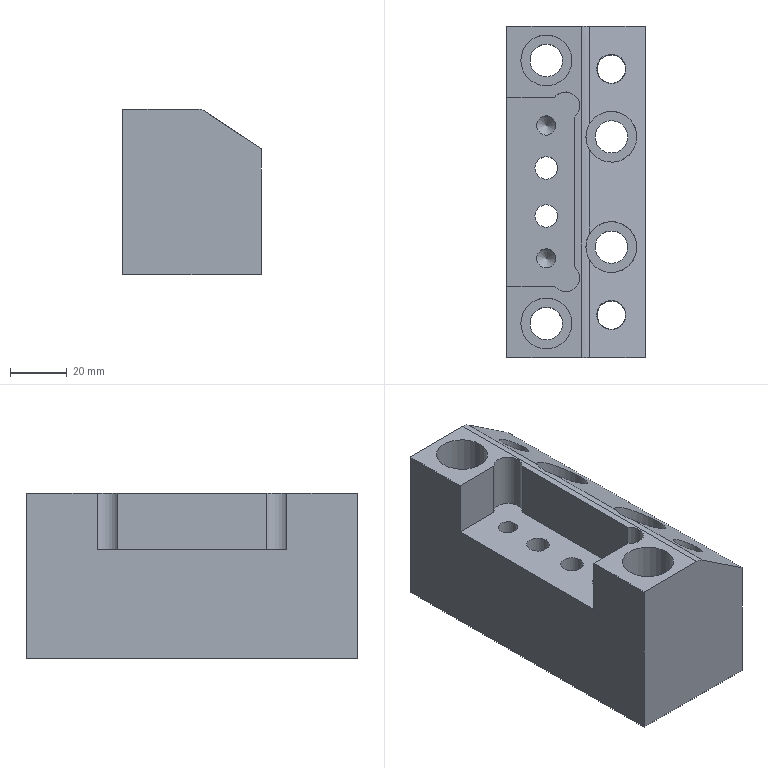Part | NX | features solid 2 | 1 solid | 42 faces | box 49 x 117 x 58.5 mm | volume 232068 mm3 | cylinder 21 | plane 19 | cone 2 | commonest cylinder face diameters 10 x5 11.5 x4 18 x4 6.8 x2 8.001 x2 10.001 x2
STEP:
#1=CARTESIAN_POINT('',(808.728,40.375,-5.567));
#2=VERTEX_POINT('',#1);
#3=CARTESIAN_POINT('',(813.878,40.375,-9.));
#4=DIRECTION('',(-0.5547,0.,-0.8321));
#5=DIRECTION('',(-0.8321,0.,0.5547));
#6=AXIS2_PLACEMENT_3D('',#3,#4,#5);
#7=ELLIPSE('',#6,6.19,5.15);
#8=EDGE_CURVE('',#2,#2,#7,.F.);
#9=ORIENTED_EDGE('',*,*,#8,.T.);
#10=EDGE_LOOP('',(#9));
#11=FACE_BOUND('',#10,.T.);
#12=CARTESIAN_POINT('',(808.728,40.375,-31.5));
#13=VERTEX_POINT('',#12);
#14=CARTESIAN_POINT('',(813.878,40.375,-31.5));
#15=DIRECTION('',(0.,0.,-1.));
#16=DIRECTION('',(-1.,0.,0.));
#17=AXIS2_PLACEMENT_3D('',#14,#15,#16);
#18=CIRCLE('',#17,5.15);
#19=EDGE_CURVE('',#13,#13,#18,.T.);
#20=ORIENTED_EDGE('',*,*,#19,.T.);
#21=EDGE_LOOP('',(#20));
#22=FACE_BOUND('',#21,.T.);
#23=CARTESIAN_POINT('',(813.878,40.375,-31.5));
#24=DIRECTION('',(0.,0.,1.));
#25=DIRECTION('',(1.,0.,0.));
#26=AXIS2_PLACEMENT_3D('',#23,#24,#25);
#27=CYLINDRICAL_SURFACE('',#26,5.15);
#28=ADVANCED_FACE('',(#11,#22),#27,.F.);
#29=ORIENTED_EDGE('',*,*,#19,.F.);
#30=EDGE_LOOP('',(#29));
#31=FACE_BOUND('',#30,.T.);
#32=CARTESIAN_POINT('',(808.877,40.375,-31.5));
#33=VERTEX_POINT('',#32);
#34=CARTESIAN_POINT('',(813.878,40.375,-31.5));
#35=DIRECTION('',(0.,0.,-1.));
#36=DIRECTION('',(-1.,0.,0.));
#37=AXIS2_PLACEMENT_3D('',#34,#35,#36);
#38=CIRCLE('',#37,5.);
#39=EDGE_CURVE('',#33,#33,#38,.F.);
#40=ORIENTED_EDGE('',*,*,#39,.F.);
#41=EDGE_LOOP('',(#40));
#42=FACE_BOUND('',#41,.T.);
#43=CARTESIAN_POINT('',(813.878,40.375,-31.5));
#44=DIRECTION('',(0.,0.,-1.));
#45=DIRECTION('',(-1.,0.,0.));
#46=AXIS2_PLACEMENT_3D('',#43,#44,#45);
#47=PLANE('',#46);
#48=ADVANCED_FACE('',(#31,#42),#47,.F.);
#49=CARTESIAN_POINT('',(795.878,5.375,-61.5));
#50=VERTEX_POINT('',#49);
#51=CARTESIAN_POINT('',(790.878,5.375,-61.5));
#52=DIRECTION('',(0.,0.,1.));
#53=DIRECTION('',(1.,0.,0.));
#54=AXIS2_PLACEMENT_3D('',#51,#52,#53);
#55=CIRCLE('',#54,5.);
#56=EDGE_CURVE('',#50,#50,#55,.F.);
#57=ORIENTED_EDGE('',*,*,#56,.F.);
#58=EDGE_LOOP('',(#57));
#59=FACE_BOUND('',#58,.T.);
#60=CARTESIAN_POINT('',(795.878,-11.625,-61.5));
#61=VERTEX_POINT('',#60);
#62=CARTESIAN_POINT('',(790.878,-11.625,-61.5));
#63=DIRECTION('',(0.,0.,1.));
#64=DIRECTION('',(1.,0.,0.));
#65=AXIS2_PLACEMENT_3D('',#62,#63,#64);
#66=CIRCLE('',#65,5.);
#67=EDGE_CURVE('',#61,#61,#66,.F.);
#68=ORIENTED_EDGE('',*,*,#67,.F.);
#69=EDGE_LOOP('',(#68));
#70=FACE_BOUND('',#69,.T.);
#71=CARTESIAN_POINT('',(819.628,-22.625,-61.5));
#72=VERTEX_POINT('',#71);
#73=CARTESIAN_POINT('',(813.878,-22.625,-61.5));
#74=DIRECTION('',(0.,0.,1.));
#75=DIRECTION('',(1.,0.,0.));
#76=AXIS2_PLACEMENT_3D('',#73,#74,#75);
#77=CIRCLE('',#76,5.75);
#78=EDGE_CURVE('',#72,#72,#77,.T.);
#79=ORIENTED_EDGE('',*,*,#78,.T.);
#80=EDGE_LOOP('',(#79));
#81=FACE_BOUND('',#80,.T.);
#82=CARTESIAN_POINT('',(796.628,43.375,-61.5));
#83=VERTEX_POINT('',#82);
#84=CARTESIAN_POINT('',(790.878,43.375,-61.5));
#85=DIRECTION('',(0.,0.,1.));
#86=DIRECTION('',(1.,0.,0.));
#87=AXIS2_PLACEMENT_3D('',#84,#85,#86);
#88=CIRCLE('',#87,5.75);
#89=EDGE_CURVE('',#83,#83,#88,.F.);
#90=ORIENTED_EDGE('',*,*,#89,.F.);
#91=EDGE_LOOP('',(#90));
#92=FACE_BOUND('',#91,.T.);
#93=CARTESIAN_POINT('',(818.878,40.375,-61.5));
#94=VERTEX_POINT('',#93);
#95=CARTESIAN_POINT('',(813.878,40.375,-61.5));
#96=DIRECTION('',(0.,0.,1.));
#97=DIRECTION('',(1.,0.,0.));
#98=AXIS2_PLACEMENT_3D('',#95,#96,#97);
#99=CIRCLE('',#98,5.);
#100=EDGE_CURVE('',#94,#94,#99,.F.);
#101=ORIENTED_EDGE('',*,*,#100,.F.);
#102=EDGE_LOOP('',(#101));
#103=FACE_BOUND('',#102,.T.);
#104=CARTESIAN_POINT('',(819.628,16.375,-61.5));
#105=VERTEX_POINT('',#104);
#106=CARTESIAN_POINT('',(813.878,16.375,-61.5));
#107=DIRECTION('',(0.,0.,1.));
#108=DIRECTION('',(1.,0.,0.));
#109=AXIS2_PLACEMENT_3D('',#106,#107,#108);
#110=CIRCLE('',#109,5.75);
#111=EDGE_CURVE('',#105,#105,#110,.F.);
#112=ORIENTED_EDGE('',*,*,#111,.F.);
#113=EDGE_LOOP('',(#112));
#114=FACE_BOUND('',#113,.T.);
#115=CARTESIAN_POINT('',(825.878,55.375,-61.5));
#116=VERTEX_POINT('',#115);
#117=CARTESIAN_POINT('',(825.878,-61.625,-61.5));
#118=VERTEX_POINT('',#117);
#119=CARTESIAN_POINT('',(825.878,0.,-61.5));
#120=DIRECTION('',(0.,1.,0.));
#121=VECTOR('',#120,1000.);
#122=LINE('',#119,#121);
#123=EDGE_CURVE('',#116,#118,#122,.F.);
#124=ORIENTED_EDGE('',*,*,#123,.T.);
#125=CARTESIAN_POINT('',(776.878,-61.625,-61.5));
#126=VERTEX_POINT('',#125);
#127=CARTESIAN_POINT('',(426.,-61.625,-61.5));
#128=DIRECTION('',(1.,0.,0.));
#129=VECTOR('',#128,1000.);
#130=LINE('',#127,#129);
#131=EDGE_CURVE('',#118,#126,#130,.F.);
#132=ORIENTED_EDGE('',*,*,#131,.T.);
#133=CARTESIAN_POINT('',(776.878,55.375,-61.5));
#134=VERTEX_POINT('',#133);
#135=CARTESIAN_POINT('',(776.878,0.,-61.5));
#136=DIRECTION('',(0.,1.,0.));
#137=VECTOR('',#136,1000.);
#138=LINE('',#135,#137);
#139=EDGE_CURVE('',#134,#126,#138,.F.);
#140=ORIENTED_EDGE('',*,*,#139,.F.);
#141=CARTESIAN_POINT('',(426.,55.375,-61.5));
#142=DIRECTION('',(1.,0.,0.));
#143=VECTOR('',#142,1000.);
#144=LINE('',#141,#143);
#145=EDGE_CURVE('',#116,#134,#144,.F.);
#146=ORIENTED_EDGE('',*,*,#145,.F.);
#147=EDGE_LOOP('',(#124,#132,#140,#146));
#148=FACE_BOUND('',#147,.T.);
#149=CARTESIAN_POINT('',(818.878,-46.625,-61.5));
#150=VERTEX_POINT('',#149);
#151=CARTESIAN_POINT('',(813.878,-46.625,-61.5));
#152=DIRECTION('',(0.,0.,1.));
#153=DIRECTION('',(1.,0.,0.));
#154=AXIS2_PLACEMENT_3D('',#151,#152,#153);
#155=CIRCLE('',#154,5.);
#156=EDGE_CURVE('',#150,#150,#155,.F.);
#157=ORIENTED_EDGE('',*,*,#156,.F.);
#158=EDGE_LOOP('',(#157));
#159=FACE_BOUND('',#158,.T.);
#160=CARTESIAN_POINT('',(796.628,-49.625,-61.5));
#161=VERTEX_POINT('',#160);
#162=CARTESIAN_POINT('',(790.878,-49.625,-61.5));
#163=DIRECTION('',(0.,0.,1.));
#164=DIRECTION('',(1.,0.,0.));
#165=AXIS2_PLACEMENT_3D('',#162,#163,#164);
#166=CIRCLE('',#165,5.75);
#167=EDGE_CURVE('',#161,#161,#166,.T.);
#168=ORIENTED_EDGE('',*,*,#167,.T.);
#169=EDGE_LOOP('',(#168));
#170=FACE_BOUND('',#169,.T.);
#171=CARTESIAN_POINT('',(426.,0.,-61.5));
#172=DIRECTION('',(0.,0.,1.));
#173=DIRECTION('',(1.,0.,0.));
#174=AXIS2_PLACEMENT_3D('',#171,#172,#173);
#175=PLANE('',#174);
#176=ADVANCED_FACE('',(#59,#70,#81,#92,#103,#114,#148,#159,#170),#175,.F.);
#177=CARTESIAN_POINT('',(799.878,-49.625,-3.));
#178=VERTEX_POINT('',#177);
#179=CARTESIAN_POINT('',(790.878,-49.625,-3.));
#180=DIRECTION('',(0.,0.,-1.));
#181=DIRECTION('',(1.,0.,0.));
#182=AXIS2_PLACEMENT_3D('',#179,#180,#181);
#183=CIRCLE('',#182,9.);
#184=EDGE_CURVE('',#178,#178,#183,.T.);
#185=ORIENTED_EDGE('',*,*,#184,.T.);
#186=EDGE_LOOP('',(#185));
#187=FACE_BOUND('',#186,.T.);
#188=CARTESIAN_POINT('',(803.364,-61.625,-3.));
#189=VERTEX_POINT('',#188);
#190=CARTESIAN_POINT('',(803.364,55.375,-3.));
#191=VERTEX_POINT('',#190);
#192=CARTESIAN_POINT('',(803.364,0.,-3.));
#193=DIRECTION('',(0.,1.,0.));
#194=VECTOR('',#193,1000.);
#195=LINE('',#192,#194);
#196=EDGE_CURVE('',#189,#191,#195,.T.);
#197=ORIENTED_EDGE('',*,*,#196,.T.);
#198=CARTESIAN_POINT('',(776.878,55.375,-3.));
#199=VERTEX_POINT('',#198);
#200=CARTESIAN_POINT('',(815.878,55.375,-3.));
#201=DIRECTION('',(-1.,0.,0.));
#202=VECTOR('',#201,1000.);
#203=LINE('',#200,#202);
#204=EDGE_CURVE('',#191,#199,#203,.T.);
#205=ORIENTED_EDGE('',*,*,#204,.T.);
#206=CARTESIAN_POINT('',(776.878,30.375,-3.));
#207=VERTEX_POINT('',#206);
#208=CARTESIAN_POINT('',(776.878,0.,-3.));
#209=DIRECTION('',(0.,-1.,0.));
#210=VECTOR('',#209,1000.);
#211=LINE('',#208,#210);
#212=EDGE_CURVE('',#199,#207,#211,.T.);
#213=ORIENTED_EDGE('',*,*,#212,.T.);
#214=CARTESIAN_POINT('',(793.839,30.375,-3.));
#215=VERTEX_POINT('',#214);
#216=CARTESIAN_POINT('',(815.878,30.375,-3.));
#217=DIRECTION('',(-1.,0.,0.));
#218=VECTOR('',#217,1000.);
#219=LINE('',#216,#218);
#220=EDGE_CURVE('',#215,#207,#219,.T.);
#221=ORIENTED_EDGE('',*,*,#220,.F.);
#222=CARTESIAN_POINT('',(800.878,23.336,-3.));
#223=VERTEX_POINT('',#222);
#224=CARTESIAN_POINT('',(797.696,27.193,-3.));
#225=DIRECTION('',(0.,0.,-1.));
#226=DIRECTION('',(-1.,0.,0.));
#227=AXIS2_PLACEMENT_3D('',#224,#225,#226);
#228=CIRCLE('',#227,5.);
#229=EDGE_CURVE('',#215,#223,#228,.T.);
#230=ORIENTED_EDGE('',*,*,#229,.T.);
#231=CARTESIAN_POINT('',(800.878,-29.586,-3.));
#232=VERTEX_POINT('',#231);
#233=CARTESIAN_POINT('',(800.878,0.,-3.));
#234=DIRECTION('',(0.,-1.,0.));
#235=VECTOR('',#234,1000.);
#236=LINE('',#233,#235);
#237=EDGE_CURVE('',#223,#232,#236,.T.);
#238=ORIENTED_EDGE('',*,*,#237,.T.);
#239=CARTESIAN_POINT('',(793.839,-36.625,-3.));
#240=VERTEX_POINT('',#239);
#241=CARTESIAN_POINT('',(797.696,-33.443,-3.));
#242=DIRECTION('',(0.,0.,-1.));
#243=DIRECTION('',(-1.,0.,0.));
#244=AXIS2_PLACEMENT_3D('',#241,#242,#243);
#245=CIRCLE('',#244,5.);
#246=EDGE_CURVE('',#232,#240,#245,.T.);
#247=ORIENTED_EDGE('',*,*,#246,.T.);
#248=CARTESIAN_POINT('',(776.878,-36.625,-3.));
#249=VERTEX_POINT('',#248);
#250=CARTESIAN_POINT('',(815.878,-36.625,-3.));
#251=DIRECTION('',(-1.,0.,0.));
#252=VECTOR('',#251,1000.);
#253=LINE('',#250,#252);
#254=EDGE_CURVE('',#240,#249,#253,.T.);
#255=ORIENTED_EDGE('',*,*,#254,.T.);
#256=CARTESIAN_POINT('',(776.878,-61.625,-3.));
#257=VERTEX_POINT('',#256);
#258=CARTESIAN_POINT('',(776.878,0.,-3.));
#259=DIRECTION('',(0.,-1.,0.));
#260=VECTOR('',#259,1000.);
#261=LINE('',#258,#260);
#262=EDGE_CURVE('',#249,#257,#261,.T.);
#263=ORIENTED_EDGE('',*,*,#262,.T.);
#264=CARTESIAN_POINT('',(815.878,-61.625,-3.));
#265=DIRECTION('',(-1.,0.,0.));
#266=VECTOR('',#265,1000.);
#267=LINE('',#264,#266);
#268=EDGE_CURVE('',#189,#257,#267,.T.);
#269=ORIENTED_EDGE('',*,*,#268,.F.);
#270=EDGE_LOOP('',(#197,#205,#213,#221,#230,#238,#247,#255,#263,#269));
#271=FACE_BOUND('',#270,.T.);
#272=CARTESIAN_POINT('',(799.878,43.375,-3.));
#273=VERTEX_POINT('',#272);
#274=CARTESIAN_POINT('',(790.878,43.375,-3.));
#275=DIRECTION('',(0.,0.,1.));
#276=DIRECTION('',(1.,0.,0.));
#277=AXIS2_PLACEMENT_3D('',#274,#275,#276);
#278=CIRCLE('',#277,9.);
#279=EDGE_CURVE('',#273,#273,#278,.T.);
#280=ORIENTED_EDGE('',*,*,#279,.F.);
#281=EDGE_LOOP('',(#280));
#282=FACE_BOUND('',#281,.T.);
#283=CARTESIAN_POINT('',(815.878,0.,-3.));
#284=DIRECTION('',(0.,0.,-1.));
#285=DIRECTION('',(-1.,0.,0.));
#286=AXIS2_PLACEMENT_3D('',#283,#284,#285);
#287=PLANE('',#286);
#288=ADVANCED_FACE('',(#187,#271,#282),#287,.F.);
#289=CARTESIAN_POINT('',(800.878,-29.586,-23.));
#290=VERTEX_POINT('',#289);
#291=CARTESIAN_POINT('',(800.878,-29.586,-23.));
#292=DIRECTION('',(0.,0.,1.));
#293=VECTOR('',#292,1000.);
#294=LINE('',#291,#293);
#295=EDGE_CURVE('',#232,#290,#294,.F.);
#296=ORIENTED_EDGE('',*,*,#295,.F.);
#297=ORIENTED_EDGE('',*,*,#237,.F.);
#298=CARTESIAN_POINT('',(800.878,23.336,-23.));
#299=VERTEX_POINT('',#298);
#300=CARTESIAN_POINT('',(800.878,23.336,-23.));
#301=DIRECTION('',(0.,0.,1.));
#302=VECTOR('',#301,1000.);
#303=LINE('',#300,#302);
#304=EDGE_CURVE('',#299,#223,#303,.T.);
#305=ORIENTED_EDGE('',*,*,#304,.F.);
#306=CARTESIAN_POINT('',(800.878,0.,-23.));
#307=DIRECTION('',(0.,-1.,0.));
#308=VECTOR('',#307,1000.);
#309=LINE('',#306,#308);
#310=EDGE_CURVE('',#299,#290,#309,.T.);
#311=ORIENTED_EDGE('',*,*,#310,.T.);
#312=EDGE_LOOP('',(#296,#297,#305,#311));
#313=FACE_BOUND('',#312,.T.);
#314=CARTESIAN_POINT('',(800.878,0.,-63.));
#315=DIRECTION('',(-1.,0.,0.));
#316=DIRECTION('',(0.,0.,1.));
#317=AXIS2_PLACEMENT_3D('',#314,#315,#316);
#318=PLANE('',#317);
#319=ADVANCED_FACE('',(#313),#318,.T.);
#320=CARTESIAN_POINT('',(825.878,55.375,-17.));
#321=VERTEX_POINT('',#320);
#322=CARTESIAN_POINT('',(825.878,55.375,-63.));
#323=DIRECTION('',(0.,0.,1.));
#324=VECTOR('',#323,1000.);
#325=LINE('',#322,#324);
#326=EDGE_CURVE('',#116,#321,#325,.T.);
#327=ORIENTED_EDGE('',*,*,#326,.T.);
#328=CARTESIAN_POINT('',(825.878,-61.625,-17.));
#329=VERTEX_POINT('',#328);
#330=CARTESIAN_POINT('',(825.878,0.,-17.));
#331=DIRECTION('',(0.,-1.,0.));
#332=VECTOR('',#331,1000.);
#333=LINE('',#330,#332);
#334=EDGE_CURVE('',#321,#329,#333,.T.);
#335=ORIENTED_EDGE('',*,*,#334,.T.);
#336=CARTESIAN_POINT('',(825.878,-61.625,-63.));
#337=DIRECTION('',(0.,0.,1.));
#338=VECTOR('',#337,1000.);
#339=LINE('',#336,#338);
#340=EDGE_CURVE('',#118,#329,#339,.T.);
#341=ORIENTED_EDGE('',*,*,#340,.F.);
#342=ORIENTED_EDGE('',*,*,#123,.F.);
#343=EDGE_LOOP('',(#327,#335,#341,#342));
#344=FACE_BOUND('',#343,.T.);
#345=CARTESIAN_POINT('',(825.878,0.,-63.));
#346=DIRECTION('',(-1.,0.,0.));
#347=DIRECTION('',(0.,0.,1.));
#348=AXIS2_PLACEMENT_3D('',#345,#346,#347);
#349=PLANE('',#348);
#350=ADVANCED_FACE('',(#344),#349,.F.);
#351=CARTESIAN_POINT('',(776.878,30.375,-23.));
#352=VERTEX_POINT('',#351);
#353=CARTESIAN_POINT('',(776.878,-36.625,-23.));
#354=VERTEX_POINT('',#353);
#355=CARTESIAN_POINT('',(776.878,0.,-23.));
#356=DIRECTION('',(0.,-1.,0.));
#357=VECTOR('',#356,1000.);
#358=LINE('',#355,#357);
#359=EDGE_CURVE('',#352,#354,#358,.T.);
#360=ORIENTED_EDGE('',*,*,#359,.F.);
#361=CARTESIAN_POINT('',(776.878,30.375,-63.));
#362=DIRECTION('',(0.,0.,1.));
#363=VECTOR('',#362,1000.);
#364=LINE('',#361,#363);
#365=EDGE_CURVE('',#352,#207,#364,.T.);
#366=ORIENTED_EDGE('',*,*,#365,.T.);
#367=ORIENTED_EDGE('',*,*,#212,.F.);
#368=CARTESIAN_POINT('',(776.878,55.375,-63.));
#369=DIRECTION('',(0.,0.,1.));
#370=VECTOR('',#369,1000.);
#371=LINE('',#368,#370);
#372=EDGE_CURVE('',#134,#199,#371,.T.);
#373=ORIENTED_EDGE('',*,*,#372,.F.);
#374=ORIENTED_EDGE('',*,*,#139,.T.);
#375=CARTESIAN_POINT('',(776.878,-61.625,-63.));
#376=DIRECTION('',(0.,0.,1.));
#377=VECTOR('',#376,1000.);
#378=LINE('',#375,#377);
#379=EDGE_CURVE('',#126,#257,#378,.T.);
#380=ORIENTED_EDGE('',*,*,#379,.T.);
#381=ORIENTED_EDGE('',*,*,#262,.F.);
#382=CARTESIAN_POINT('',(776.878,-36.625,-63.));
#383=DIRECTION('',(0.,0.,1.));
#384=VECTOR('',#383,1000.);
#385=LINE('',#382,#384);
#386=EDGE_CURVE('',#354,#249,#385,.T.);
#387=ORIENTED_EDGE('',*,*,#386,.F.);
#388=EDGE_LOOP('',(#360,#366,#367,#373,#374,#380,#381,#387));
#389=FACE_BOUND('',#388,.T.);
#390=CARTESIAN_POINT('',(776.878,0.,-63.));
#391=DIRECTION('',(-1.,0.,0.));
#392=DIRECTION('',(0.,0.,1.));
#393=AXIS2_PLACEMENT_3D('',#390,#391,#392);
#394=PLANE('',#393);
#395=ADVANCED_FACE('',(#389),#394,.T.);
#396=CARTESIAN_POINT('',(794.278,20.375,-23.));
#397=VERTEX_POINT('',#396);
#398=CARTESIAN_POINT('',(790.878,20.375,-23.));
#399=DIRECTION('',(0.,0.,-1.));
#400=DIRECTION('',(1.,0.,0.));
#401=AXIS2_PLACEMENT_3D('',#398,#399,#400);
#402=CIRCLE('',#401,3.4);
#403=EDGE_CURVE('',#397,#397,#402,.T.);
#404=ORIENTED_EDGE('',*,*,#403,.T.);
#405=EDGE_LOOP('',(#404));
#406=FACE_BOUND('',#405,.T.);
#407=CARTESIAN_POINT('',(794.278,-26.625,-23.));
#408=VERTEX_POINT('',#407);
#409=CARTESIAN_POINT('',(790.878,-26.625,-23.));
#410=DIRECTION('',(0.,0.,-1.));
#411=DIRECTION('',(1.,0.,0.));
#412=AXIS2_PLACEMENT_3D('',#409,#410,#411);
#413=CIRCLE('',#412,3.4);
#414=EDGE_CURVE('',#408,#408,#413,.T.);
#415=ORIENTED_EDGE('',*,*,#414,.T.);
#416=EDGE_LOOP('',(#415));
#417=FACE_BOUND('',#416,.T.);
#418=CARTESIAN_POINT('',(794.878,5.375,-23.));
#419=VERTEX_POINT('',#418);
#420=CARTESIAN_POINT('',(790.878,5.375,-23.));
#421=DIRECTION('',(0.,0.,-1.));
#422=DIRECTION('',(1.,0.,0.));
#423=AXIS2_PLACEMENT_3D('',#420,#421,#422);
#424=CIRCLE('',#423,4.);
#425=EDGE_CURVE('',#419,#419,#424,.T.);
#426=ORIENTED_EDGE('',*,*,#425,.T.);
#427=EDGE_LOOP('',(#426));
#428=FACE_BOUND('',#427,.T.);
#429=CARTESIAN_POINT('',(794.878,-11.625,-23.));
#430=VERTEX_POINT('',#429);
#431=CARTESIAN_POINT('',(790.878,-11.625,-23.));
#432=DIRECTION('',(0.,0.,-1.));
#433=DIRECTION('',(1.,0.,0.));
#434=AXIS2_PLACEMENT_3D('',#431,#432,#433);
#435=CIRCLE('',#434,4.);
#436=EDGE_CURVE('',#430,#430,#435,.T.);
#437=ORIENTED_EDGE('',*,*,#436,.T.);
#438=EDGE_LOOP('',(#437));
#439=FACE_BOUND('',#438,.T.);
#440=CARTESIAN_POINT('',(793.839,-36.625,-23.));
#441=VERTEX_POINT('',#440);
#442=CARTESIAN_POINT('',(797.696,-33.443,-23.));
#443=DIRECTION('',(0.,0.,1.));
#444=DIRECTION('',(1.,0.,0.));
#445=AXIS2_PLACEMENT_3D('',#442,#443,#444);
#446=CIRCLE('',#445,5.);
#447=EDGE_CURVE('',#441,#290,#446,.T.);
#448=ORIENTED_EDGE('',*,*,#447,.T.);
#449=ORIENTED_EDGE('',*,*,#310,.F.);
#450=CARTESIAN_POINT('',(793.839,30.375,-23.));
#451=VERTEX_POINT('',#450);
#452=CARTESIAN_POINT('',(797.696,27.193,-23.));
#453=DIRECTION('',(0.,0.,1.));
#454=DIRECTION('',(1.,0.,0.));
#455=AXIS2_PLACEMENT_3D('',#452,#453,#454);
#456=CIRCLE('',#455,5.);
#457=EDGE_CURVE('',#299,#451,#456,.T.);
#458=ORIENTED_EDGE('',*,*,#457,.T.);
#459=CARTESIAN_POINT('',(699.237,30.375,-23.));
#460=DIRECTION('',(-1.,0.,0.));
#461=VECTOR('',#460,1000.);
#462=LINE('',#459,#461);
#463=EDGE_CURVE('',#451,#352,#462,.T.);
#464=ORIENTED_EDGE('',*,*,#463,.T.);
#465=ORIENTED_EDGE('',*,*,#359,.T.);
#466=CARTESIAN_POINT('',(699.237,-36.625,-23.));
#467=DIRECTION('',(-1.,0.,0.));
#468=VECTOR('',#467,1000.);
#469=LINE('',#466,#468);
#470=EDGE_CURVE('',#441,#354,#469,.T.);
#471=ORIENTED_EDGE('',*,*,#470,.F.);
#472=EDGE_LOOP('',(#448,#449,#458,#464,#465,#471));
#473=FACE_BOUND('',#472,.T.);
#474=CARTESIAN_POINT('',(699.237,0.,-23.));
#475=DIRECTION('',(0.,0.,-1.));
#476=DIRECTION('',(-1.,0.,0.));
#477=AXIS2_PLACEMENT_3D('',#474,#475,#476);
#478=PLANE('',#477);
#479=ADVANCED_FACE('',(#406,#417,#428,#439,#473),#478,.F.);
#480=CARTESIAN_POINT('',(806.137,-61.625,-3.84));
#481=VERTEX_POINT('',#480);
#482=CARTESIAN_POINT('',(840.185,-61.625,-26.538));
#483=DIRECTION('',(0.8321,0.,-0.5547));
#484=VECTOR('',#483,1000.);
#485=LINE('',#482,#484);
#486=EDGE_CURVE('',#329,#481,#485,.F.);
#487=ORIENTED_EDGE('',*,*,#486,.T.);
#488=CARTESIAN_POINT('',(803.364,-61.625,-8.));
#489=DIRECTION('',(0.,-1.,0.));
#490=DIRECTION('',(0.,0.,-1.));
#491=AXIS2_PLACEMENT_3D('',#488,#489,#490);
#492=CIRCLE('',#491,5.);
#493=EDGE_CURVE('',#481,#189,#492,.T.);
#494=ORIENTED_EDGE('',*,*,#493,.T.);
#495=ORIENTED_EDGE('',*,*,#268,.T.);
#496=ORIENTED_EDGE('',*,*,#379,.F.);
#497=ORIENTED_EDGE('',*,*,#131,.F.);
#498=ORIENTED_EDGE('',*,*,#340,.T.);
#499=EDGE_LOOP('',(#487,#494,#495,#496,#497,#498));
#500=FACE_BOUND('',#499,.T.);
#501=CARTESIAN_POINT('',(815.878,-61.625,-63.));
#502=DIRECTION('',(0.,-1.,0.));
#503=DIRECTION('',(0.,0.,-1.));
#504=AXIS2_PLACEMENT_3D('',#501,#502,#503);
#505=PLANE('',#504);
#506=ADVANCED_FACE('',(#500),#505,.T.);
#507=ORIENTED_EDGE('',*,*,#254,.F.);
#508=CARTESIAN_POINT('',(793.839,-36.625,-23.));
#509=DIRECTION('',(0.,0.,1.));
#510=VECTOR('',#509,1000.);
#511=LINE('',#508,#510);
#512=EDGE_CURVE('',#240,#441,#511,.F.);
#513=ORIENTED_EDGE('',*,*,#512,.T.);
#514=ORIENTED_EDGE('',*,*,#470,.T.);
#515=ORIENTED_EDGE('',*,*,#386,.T.);
#516=EDGE_LOOP('',(#507,#513,#514,#515));
#517=FACE_BOUND('',#516,.T.);
#518=CARTESIAN_POINT('',(815.878,-36.625,-63.));
#519=DIRECTION('',(0.,-1.,0.));
#520=DIRECTION('',(0.,0.,-1.));
#521=AXIS2_PLACEMENT_3D('',#518,#519,#520);
#522=PLANE('',#521);
#523=ADVANCED_FACE('',(#517),#522,.F.);
#524=CARTESIAN_POINT('',(793.839,30.375,-23.));
#525=DIRECTION('',(0.,0.,1.));
#526=VECTOR('',#525,1000.);
#527=LINE('',#524,#526);
#528=EDGE_CURVE('',#215,#451,#527,.F.);
#529=ORIENTED_EDGE('',*,*,#528,.F.);
#530=ORIENTED_EDGE('',*,*,#220,.T.);
#531=ORIENTED_EDGE('',*,*,#365,.F.);
#532=ORIENTED_EDGE('',*,*,#463,.F.);
#533=EDGE_LOOP('',(#529,#530,#531,#532));
#534=FACE_BOUND('',#533,.T.);
#535=CARTESIAN_POINT('',(815.878,30.375,-63.));
#536=DIRECTION('',(0.,-1.,0.));
#537=DIRECTION('',(0.,0.,-1.));
#538=AXIS2_PLACEMENT_3D('',#535,#536,#537);
#539=PLANE('',#538);
#540=ADVANCED_FACE('',(#534),#539,.T.);
#541=ORIENTED_EDGE('',*,*,#204,.F.);
#542=CARTESIAN_POINT('',(806.137,55.375,-3.84));
#543=VERTEX_POINT('',#542);
#544=CARTESIAN_POINT('',(803.364,55.375,-8.));
#545=DIRECTION('',(0.,-1.,0.));
#546=DIRECTION('',(0.,0.,-1.));
#547=AXIS2_PLACEMENT_3D('',#544,#545,#546);
#548=CIRCLE('',#547,5.);
#549=EDGE_CURVE('',#191,#543,#548,.F.);
#550=ORIENTED_EDGE('',*,*,#549,.T.);
#551=CARTESIAN_POINT('',(825.878,55.375,-17.));
#552=DIRECTION('',(-0.8321,0.,0.5547));
#553=VECTOR('',#552,1000.);
#554=LINE('',#551,#553);
#555=EDGE_CURVE('',#543,#321,#554,.F.);
#556=ORIENTED_EDGE('',*,*,#555,.T.);
#557=ORIENTED_EDGE('',*,*,#326,.F.);
#558=ORIENTED_EDGE('',*,*,#145,.T.);
#559=ORIENTED_EDGE('',*,*,#372,.T.);
#560=EDGE_LOOP('',(#541,#550,#556,#557,#558,#559));
#561=FACE_BOUND('',#560,.T.);
#562=CARTESIAN_POINT('',(815.878,55.375,-63.));
#563=DIRECTION('',(0.,-1.,0.));
#564=DIRECTION('',(0.,0.,-1.));
#565=AXIS2_PLACEMENT_3D('',#562,#563,#564);
#566=PLANE('',#565);
#567=ADVANCED_FACE('',(#561),#566,.F.);
#568=ORIENTED_EDGE('',*,*,#304,.T.);
#569=ORIENTED_EDGE('',*,*,#229,.F.);
#570=ORIENTED_EDGE('',*,*,#528,.T.);
#571=ORIENTED_EDGE('',*,*,#457,.F.);
#572=EDGE_LOOP('',(#568,#569,#570,#571));
#573=FACE_BOUND('',#572,.T.);
#574=CARTESIAN_POINT('',(797.696,27.193,-23.));
#575=DIRECTION('',(0.,0.,1.));
#576=DIRECTION('',(1.,0.,0.));
#577=AXIS2_PLACEMENT_3D('',#574,#575,#576);
#578=CYLINDRICAL_SURFACE('',#577,5.);
#579=ADVANCED_FACE('',(#573),#578,.F.);
#580=ORIENTED_EDGE('',*,*,#295,.T.);
#581=ORIENTED_EDGE('',*,*,#447,.F.);
#582=ORIENTED_EDGE('',*,*,#512,.F.);
#583=ORIENTED_EDGE('',*,*,#246,.F.);
#584=EDGE_LOOP('',(#580,#581,#582,#583));
#585=FACE_BOUND('',#584,.T.);
#586=CARTESIAN_POINT('',(797.696,-33.443,-23.));
#587=DIRECTION('',(0.,0.,1.));
#588=DIRECTION('',(1.,0.,0.));
#589=AXIS2_PLACEMENT_3D('',#586,#587,#588);
#590=CYLINDRICAL_SURFACE('',#589,5.);
#591=ADVANCED_FACE('',(#585),#590,.F.);
#592=CARTESIAN_POINT('',(808.128,16.375,-31.));
#593=VERTEX_POINT('',#592);
#594=CARTESIAN_POINT('',(813.878,16.375,-31.));
#595=DIRECTION('',(0.,0.,1.));
#596=DIRECTION('',(-1.,0.,0.));
#597=AXIS2_PLACEMENT_3D('',#594,#595,#596);
#598=CIRCLE('',#597,5.75);
#599=EDGE_CURVE('',#593,#593,#598,.T.);
#600=ORIENTED_EDGE('',*,*,#599,.T.);
#601=EDGE_LOOP('',(#600));
#602=FACE_BOUND('',#601,.T.);
#603=ORIENTED_EDGE('',*,*,#111,.T.);
#604=EDGE_LOOP('',(#603));
#605=FACE_BOUND('',#604,.T.);
#606=CARTESIAN_POINT('',(813.878,16.375,-3.));
#607=DIRECTION('',(0.,0.,-1.));
#608=DIRECTION('',(1.,0.,0.));
#609=AXIS2_PLACEMENT_3D('',#606,#607,#608);
#610=CYLINDRICAL_SURFACE('',#609,5.75);
#611=ADVANCED_FACE('',(#602,#605),#610,.F.);
#612=ORIENTED_EDGE('',*,*,#599,.F.);
#613=EDGE_LOOP('',(#612));
#614=FACE_BOUND('',#613,.T.);
#615=CARTESIAN_POINT('',(822.878,16.375,-31.));
#616=VERTEX_POINT('',#615);
#617=CARTESIAN_POINT('',(813.878,16.375,-31.));
#618=DIRECTION('',(0.,0.,-1.));
#619=DIRECTION('',(1.,0.,0.));
#620=AXIS2_PLACEMENT_3D('',#617,#618,#619);
#621=CIRCLE('',#620,9.);
#622=EDGE_CURVE('',#616,#616,#621,.F.);
#623=ORIENTED_EDGE('',*,*,#622,.T.);
#624=EDGE_LOOP('',(#623));
#625=FACE_BOUND('',#624,.T.);
#626=CARTESIAN_POINT('',(813.878,16.375,-31.));
#627=DIRECTION('',(0.,0.,-1.));
#628=DIRECTION('',(-1.,0.,0.));
#629=AXIS2_PLACEMENT_3D('',#626,#627,#628);
#630=PLANE('',#629);
#631=ADVANCED_FACE('',(#614,#625),#630,.F.);
#632=ORIENTED_EDGE('',*,*,#622,.F.);
#633=EDGE_LOOP('',(#632));
#634=FACE_BOUND('',#633,.T.);
#635=CARTESIAN_POINT('',(806.137,20.967,-3.84));
#636=VERTEX_POINT('',#635);
#637=CARTESIAN_POINT('',(806.137,11.783,-3.84));
#638=VERTEX_POINT('',#637);
#639=CARTESIAN_POINT('',(806.137,20.967,-3.84));
#640=CARTESIAN_POINT('',(805.353,19.645,-3.317));
#641=CARTESIAN_POINT('',(804.406,16.344,-3.155));
#642=CARTESIAN_POINT('',(805.345,13.118,-3.312));
#643=CARTESIAN_POINT('',(806.137,11.783,-3.84));
#644=B_SPLINE_CURVE_WITH_KNOTS('',3,(#639,#640,#641,#642,#643),.UNSPECIFIED.,.F.,.F.,(4,1,4),(0.04031,0.04517,0.05002),.UNSPECIFIED.);
#645=EDGE_CURVE('',#636,#638,#644,.T.);
#646=ORIENTED_EDGE('',*,*,#645,.T.);
#647=CARTESIAN_POINT('',(813.878,16.375,-9.));
#648=DIRECTION('',(-0.5547,0.,-0.8321));
#649=DIRECTION('',(0.8321,0.,-0.5547));
#650=AXIS2_PLACEMENT_3D('',#647,#648,#649);
#651=ELLIPSE('',#650,10.817,9.);
#652=EDGE_CURVE('',#638,#636,#651,.F.);
#653=ORIENTED_EDGE('',*,*,#652,.T.);
#654=EDGE_LOOP('',(#646,#653));
#655=FACE_BOUND('',#654,.T.);
#656=CARTESIAN_POINT('',(813.878,16.375,-3.));
#657=DIRECTION('',(0.,0.,-1.));
#658=DIRECTION('',(1.,0.,0.));
#659=AXIS2_PLACEMENT_3D('',#656,#657,#658);
#660=CYLINDRICAL_SURFACE('',#659,9.);
#661=ADVANCED_FACE('',(#634,#655),#660,.F.);
#662=ORIENTED_EDGE('',*,*,#39,.T.);
#663=EDGE_LOOP('',(#662));
#664=FACE_BOUND('',#663,.T.);
#665=ORIENTED_EDGE('',*,*,#100,.T.);
#666=EDGE_LOOP('',(#665));
#667=FACE_BOUND('',#666,.T.);
#668=CARTESIAN_POINT('',(813.878,40.375,22.));
#669=DIRECTION('',(0.,0.,-1.));
#670=DIRECTION('',(-1.,0.,0.));
#671=AXIS2_PLACEMENT_3D('',#668,#669,#670);
#672=CYLINDRICAL_SURFACE('',#671,5.);
#673=ADVANCED_FACE('',(#664,#667),#672,.F.);
#674=CARTESIAN_POINT('',(785.128,43.375,-31.));
#675=VERTEX_POINT('',#674);
#676=CARTESIAN_POINT('',(790.878,43.375,-31.));
#677=DIRECTION('',(0.,0.,1.));
#678=DIRECTION('',(-1.,0.,0.));
#679=AXIS2_PLACEMENT_3D('',#676,#677,#678);
#680=CIRCLE('',#679,5.75);
#681=EDGE_CURVE('',#675,#675,#680,.T.);
#682=ORIENTED_EDGE('',*,*,#681,.T.);
#683=EDGE_LOOP('',(#682));
#684=FACE_BOUND('',#683,.T.);
#685=ORIENTED_EDGE('',*,*,#89,.T.);
#686=EDGE_LOOP('',(#685));
#687=FACE_BOUND('',#686,.T.);
#688=CARTESIAN_POINT('',(790.878,43.375,-3.));
#689=DIRECTION('',(0.,0.,-1.));
#690=DIRECTION('',(1.,0.,0.));
#691=AXIS2_PLACEMENT_3D('',#688,#689,#690);
#692=CYLINDRICAL_SURFACE('',#691,5.75);
#693=ADVANCED_FACE('',(#684,#687),#692,.F.);
#694=ORIENTED_EDGE('',*,*,#681,.F.);
#695=EDGE_LOOP('',(#694));
#696=FACE_BOUND('',#695,.T.);
#697=CARTESIAN_POINT('',(799.878,43.375,-31.));
#698=VERTEX_POINT('',#697);
#699=CARTESIAN_POINT('',(790.878,43.375,-31.));
#700=DIRECTION('',(0.,0.,-1.));
#701=DIRECTION('',(1.,0.,0.));
#702=AXIS2_PLACEMENT_3D('',#699,#700,#701);
#703=CIRCLE('',#702,9.);
#704=EDGE_CURVE('',#698,#698,#703,.F.);
#705=ORIENTED_EDGE('',*,*,#704,.T.);
#706=EDGE_LOOP('',(#705));
#707=FACE_BOUND('',#706,.T.);
#708=CARTESIAN_POINT('',(790.878,43.375,-31.));
#709=DIRECTION('',(0.,0.,-1.));
#710=DIRECTION('',(-1.,0.,0.));
#711=AXIS2_PLACEMENT_3D('',#708,#709,#710);
#712=PLANE('',#711);
#713=ADVANCED_FACE('',(#696,#707),#712,.F.);
#714=ORIENTED_EDGE('',*,*,#704,.F.);
#715=EDGE_LOOP('',(#714));
#716=FACE_BOUND('',#715,.T.);
#717=ORIENTED_EDGE('',*,*,#279,.T.);
#718=EDGE_LOOP('',(#717));
#719=FACE_BOUND('',#718,.T.);
#720=CARTESIAN_POINT('',(790.878,43.375,-3.));
#721=DIRECTION('',(0.,0.,-1.));
#722=DIRECTION('',(1.,0.,0.));
#723=AXIS2_PLACEMENT_3D('',#720,#721,#722);
#724=CYLINDRICAL_SURFACE('',#723,9.);
#725=ADVANCED_FACE('',(#716,#719),#724,.F.);
#726=CARTESIAN_POINT('',(808.128,-22.625,-31.));
#727=VERTEX_POINT('',#726);
#728=CARTESIAN_POINT('',(813.878,-22.625,-31.));
#729=DIRECTION('',(0.,0.,-1.));
#730=DIRECTION('',(-1.,0.,0.));
#731=AXIS2_PLACEMENT_3D('',#728,#729,#730);
#732=CIRCLE('',#731,5.75);
#733=EDGE_CURVE('',#727,#727,#732,.T.);
#734=ORIENTED_EDGE('',*,*,#733,.F.);
#735=EDGE_LOOP('',(#734));
#736=FACE_BOUND('',#735,.T.);
#737=ORIENTED_EDGE('',*,*,#78,.F.);
#738=EDGE_LOOP('',(#737));
#739=FACE_BOUND('',#738,.T.);
#740=CARTESIAN_POINT('',(813.878,-22.625,-3.));
#741=DIRECTION('',(0.,0.,-1.));
#742=DIRECTION('',(1.,0.,0.));
#743=AXIS2_PLACEMENT_3D('',#740,#741,#742);
#744=CYLINDRICAL_SURFACE('',#743,5.75);
#745=ADVANCED_FACE('',(#736,#739),#744,.F.);
#746=ORIENTED_EDGE('',*,*,#733,.T.);
#747=EDGE_LOOP('',(#746));
#748=FACE_BOUND('',#747,.T.);
#749=CARTESIAN_POINT('',(822.878,-22.625,-31.));
#750=VERTEX_POINT('',#749);
#751=CARTESIAN_POINT('',(813.878,-22.625,-31.));
#752=DIRECTION('',(0.,0.,1.));
#753=DIRECTION('',(1.,0.,0.));
#754=AXIS2_PLACEMENT_3D('',#751,#752,#753);
#755=CIRCLE('',#754,9.);
#756=EDGE_CURVE('',#750,#750,#755,.F.);
#757=ORIENTED_EDGE('',*,*,#756,.F.);
#758=EDGE_LOOP('',(#757));
#759=FACE_BOUND('',#758,.T.);
#760=CARTESIAN_POINT('',(813.878,-22.625,-31.));
#761=DIRECTION('',(0.,0.,-1.));
#762=DIRECTION('',(-1.,0.,0.));
#763=AXIS2_PLACEMENT_3D('',#760,#761,#762);
#764=PLANE('',#763);
#765=ADVANCED_FACE('',(#748,#759),#764,.F.);
#766=ORIENTED_EDGE('',*,*,#756,.T.);
#767=EDGE_LOOP('',(#766));
#768=FACE_BOUND('',#767,.T.);
#769=CARTESIAN_POINT('',(806.137,-27.217,-3.84));
#770=VERTEX_POINT('',#769);
#771=CARTESIAN_POINT('',(806.137,-18.033,-3.84));
#772=VERTEX_POINT('',#771);
#773=CARTESIAN_POINT('',(806.137,-27.217,-3.84));
#774=CARTESIAN_POINT('',(805.353,-25.894,-3.317));
#775=CARTESIAN_POINT('',(804.406,-22.594,-3.155));
#776=CARTESIAN_POINT('',(805.345,-19.368,-3.312));
#777=CARTESIAN_POINT('',(806.137,-18.033,-3.84));
#778=B_SPLINE_CURVE_WITH_KNOTS('',3,(#773,#774,#775,#776,#777),.UNSPECIFIED.,.F.,.F.,(4,1,4),(0.04031,0.04517,0.05002),.UNSPECIFIED.);
#779=EDGE_CURVE('',#770,#772,#778,.T.);
#780=ORIENTED_EDGE('',*,*,#779,.F.);
#781=CARTESIAN_POINT('',(813.878,-22.625,-9.));
#782=DIRECTION('',(-0.5547,0.,-0.8321));
#783=DIRECTION('',(0.8321,0.,-0.5547));
#784=AXIS2_PLACEMENT_3D('',#781,#782,#783);
#785=ELLIPSE('',#784,10.817,9.);
#786=EDGE_CURVE('',#772,#770,#785,.T.);
#787=ORIENTED_EDGE('',*,*,#786,.F.);
#788=EDGE_LOOP('',(#780,#787));
#789=FACE_BOUND('',#788,.T.);
#790=CARTESIAN_POINT('',(813.878,-22.625,-3.));
#791=DIRECTION('',(0.,0.,-1.));
#792=DIRECTION('',(1.,0.,0.));
#793=AXIS2_PLACEMENT_3D('',#790,#791,#792);
#794=CYLINDRICAL_SURFACE('',#793,9.);
#795=ADVANCED_FACE('',(#768,#789),#794,.F.);
#796=CARTESIAN_POINT('',(808.877,-46.625,-31.5));
#797=VERTEX_POINT('',#796);
#798=CARTESIAN_POINT('',(813.878,-46.625,-31.5));
#799=DIRECTION('',(0.,0.,-1.));
#800=DIRECTION('',(-1.,0.,0.));
#801=AXIS2_PLACEMENT_3D('',#798,#799,#800);
#802=CIRCLE('',#801,5.);
#803=EDGE_CURVE('',#797,#797,#802,.F.);
#804=ORIENTED_EDGE('',*,*,#803,.T.);
#805=EDGE_LOOP('',(#804));
#806=FACE_BOUND('',#805,.T.);
#807=ORIENTED_EDGE('',*,*,#156,.T.);
#808=EDGE_LOOP('',(#807));
#809=FACE_BOUND('',#808,.T.);
#810=CARTESIAN_POINT('',(813.878,-46.625,22.));
#811=DIRECTION('',(0.,0.,-1.));
#812=DIRECTION('',(-1.,0.,0.));
#813=AXIS2_PLACEMENT_3D('',#810,#811,#812);
#814=CYLINDRICAL_SURFACE('',#813,5.);
#815=ADVANCED_FACE('',(#806,#809),#814,.F.);
#816=CARTESIAN_POINT('',(785.128,-49.625,-31.));
#817=VERTEX_POINT('',#816);
#818=CARTESIAN_POINT('',(790.878,-49.625,-31.));
#819=DIRECTION('',(0.,0.,-1.));
#820=DIRECTION('',(-1.,0.,0.));
#821=AXIS2_PLACEMENT_3D('',#818,#819,#820);
#822=CIRCLE('',#821,5.75);
#823=EDGE_CURVE('',#817,#817,#822,.T.);
#824=ORIENTED_EDGE('',*,*,#823,.F.);
#825=EDGE_LOOP('',(#824));
#826=FACE_BOUND('',#825,.T.);
#827=ORIENTED_EDGE('',*,*,#167,.F.);
#828=EDGE_LOOP('',(#827));
#829=FACE_BOUND('',#828,.T.);
#830=CARTESIAN_POINT('',(790.878,-49.625,-3.));
#831=DIRECTION('',(0.,0.,-1.));
#832=DIRECTION('',(1.,0.,0.));
#833=AXIS2_PLACEMENT_3D('',#830,#831,#832);
#834=CYLINDRICAL_SURFACE('',#833,5.75);
#835=ADVANCED_FACE('',(#826,#829),#834,.F.);
#836=ORIENTED_EDGE('',*,*,#823,.T.);
#837=EDGE_LOOP('',(#836));
#838=FACE_BOUND('',#837,.T.);
#839=CARTESIAN_POINT('',(799.878,-49.625,-31.));
#840=VERTEX_POINT('',#839);
#841=CARTESIAN_POINT('',(790.878,-49.625,-31.));
#842=DIRECTION('',(0.,0.,1.));
#843=DIRECTION('',(1.,0.,0.));
#844=AXIS2_PLACEMENT_3D('',#841,#842,#843);
#845=CIRCLE('',#844,9.);
#846=EDGE_CURVE('',#840,#840,#845,.F.);
#847=ORIENTED_EDGE('',*,*,#846,.F.);
#848=EDGE_LOOP('',(#847));
#849=FACE_BOUND('',#848,.T.);
#850=CARTESIAN_POINT('',(790.878,-49.625,-31.));
#851=DIRECTION('',(0.,0.,-1.));
#852=DIRECTION('',(-1.,0.,0.));
#853=AXIS2_PLACEMENT_3D('',#850,#851,#852);
#854=PLANE('',#853);
#855=ADVANCED_FACE('',(#838,#849),#854,.F.);
#856=ORIENTED_EDGE('',*,*,#846,.T.);
#857=EDGE_LOOP('',(#856));
#858=FACE_BOUND('',#857,.T.);
#859=ORIENTED_EDGE('',*,*,#184,.F.);
#860=EDGE_LOOP('',(#859));
#861=FACE_BOUND('',#860,.T.);
#862=CARTESIAN_POINT('',(790.878,-49.625,-3.));
#863=DIRECTION('',(0.,0.,-1.));
#864=DIRECTION('',(1.,0.,0.));
#865=AXIS2_PLACEMENT_3D('',#862,#863,#864);
#866=CYLINDRICAL_SURFACE('',#865,9.);
#867=ADVANCED_FACE('',(#858,#861),#866,.F.);
#868=ORIENTED_EDGE('',*,*,#8,.F.);
#869=EDGE_LOOP('',(#868));
#870=FACE_BOUND('',#869,.T.);
#871=CARTESIAN_POINT('',(808.728,-46.625,-5.567));
#872=VERTEX_POINT('',#871);
#873=CARTESIAN_POINT('',(813.878,-46.625,-9.));
#874=DIRECTION('',(-0.5547,0.,-0.8321));
#875=DIRECTION('',(-0.8321,0.,0.5547));
#876=AXIS2_PLACEMENT_3D('',#873,#874,#875);
#877=ELLIPSE('',#876,6.19,5.15);
#878=EDGE_CURVE('',#872,#872,#877,.F.);
#879=ORIENTED_EDGE('',*,*,#878,.F.);
#880=EDGE_LOOP('',(#879));
#881=FACE_BOUND('',#880,.T.);
#882=ORIENTED_EDGE('',*,*,#555,.F.);
#883=CARTESIAN_POINT('',(806.137,16.375,-3.84));
#884=DIRECTION('',(0.,1.,0.));
#885=VECTOR('',#884,1000.);
#886=LINE('',#883,#885);
#887=EDGE_CURVE('',#543,#636,#886,.F.);
#888=ORIENTED_EDGE('',*,*,#887,.T.);
#889=ORIENTED_EDGE('',*,*,#652,.F.);
#890=CARTESIAN_POINT('',(806.137,-22.625,-3.84));
#891=DIRECTION('',(0.,1.,0.));
#892=VECTOR('',#891,1000.);
#893=LINE('',#890,#892);
#894=EDGE_CURVE('',#638,#772,#893,.F.);
#895=ORIENTED_EDGE('',*,*,#894,.T.);
#896=ORIENTED_EDGE('',*,*,#786,.T.);
#897=CARTESIAN_POINT('',(806.137,-61.625,-3.84));
#898=DIRECTION('',(0.,1.,0.));
#899=VECTOR('',#898,1000.);
#900=LINE('',#897,#899);
#901=EDGE_CURVE('',#770,#481,#900,.F.);
#902=ORIENTED_EDGE('',*,*,#901,.T.);
#903=ORIENTED_EDGE('',*,*,#486,.F.);
#904=ORIENTED_EDGE('',*,*,#334,.F.);
#905=EDGE_LOOP('',(#882,#888,#889,#895,#896,#902,#903,#904));
#906=FACE_BOUND('',#905,.T.);
#907=CARTESIAN_POINT('',(825.878,0.,-17.));
#908=DIRECTION('',(-0.5547,0.,-0.8321));
#909=DIRECTION('',(0.,-1.,0.));
#910=AXIS2_PLACEMENT_3D('',#907,#908,#909);
#911=PLANE('',#910);
#912=ADVANCED_FACE('',(#870,#881,#906),#911,.F.);
#913=ORIENTED_EDGE('',*,*,#549,.F.);
#914=ORIENTED_EDGE('',*,*,#196,.F.);
#915=ORIENTED_EDGE('',*,*,#493,.F.);
#916=ORIENTED_EDGE('',*,*,#901,.F.);
#917=ORIENTED_EDGE('',*,*,#779,.T.);
#918=ORIENTED_EDGE('',*,*,#894,.F.);
#919=ORIENTED_EDGE('',*,*,#645,.F.);
#920=ORIENTED_EDGE('',*,*,#887,.F.);
#921=EDGE_LOOP('',(#913,#914,#915,#916,#917,#918,#919,#920));
#922=FACE_BOUND('',#921,.T.);
#923=CARTESIAN_POINT('',(803.364,0.,-8.));
#924=DIRECTION('',(0.,1.,0.));
#925=DIRECTION('',(0.,0.,1.));
#926=AXIS2_PLACEMENT_3D('',#923,#924,#925);
#927=CYLINDRICAL_SURFACE('',#926,5.);
#928=ADVANCED_FACE('',(#922),#927,.T.);
#929=CARTESIAN_POINT('',(794.878,-11.625,-48.));
#930=VERTEX_POINT('',#929);
#931=CARTESIAN_POINT('',(790.878,-11.625,-48.));
#932=DIRECTION('',(0.,0.,1.));
#933=DIRECTION('',(1.,0.,0.));
#934=AXIS2_PLACEMENT_3D('',#931,#932,#933);
#935=CIRCLE('',#934,4.);
#936=EDGE_CURVE('',#930,#930,#935,.F.);
#937=ORIENTED_EDGE('',*,*,#936,.F.);
#938=EDGE_LOOP('',(#937));
#939=FACE_BOUND('',#938,.T.);
#940=CARTESIAN_POINT('',(795.878,-11.625,-48.));
#941=VERTEX_POINT('',#940);
#942=CARTESIAN_POINT('',(790.878,-11.625,-48.));
#943=DIRECTION('',(0.,0.,-1.));
#944=DIRECTION('',(1.,0.,0.));
#945=AXIS2_PLACEMENT_3D('',#942,#943,#944);
#946=CIRCLE('',#945,5.);
#947=EDGE_CURVE('',#941,#941,#946,.F.);
#948=ORIENTED_EDGE('',*,*,#947,.F.);
#949=EDGE_LOOP('',(#948));
#950=FACE_BOUND('',#949,.T.);
#951=CARTESIAN_POINT('',(790.878,-11.625,-48.));
#952=DIRECTION('',(0.,0.,1.));
#953=DIRECTION('',(1.,0.,0.));
#954=AXIS2_PLACEMENT_3D('',#951,#952,#953);
#955=PLANE('',#954);
#956=ADVANCED_FACE('',(#939,#950),#955,.F.);
#957=ORIENTED_EDGE('',*,*,#67,.T.);
#958=EDGE_LOOP('',(#957));
#959=FACE_BOUND('',#958,.T.);
#960=ORIENTED_EDGE('',*,*,#947,.T.);
#961=EDGE_LOOP('',(#960));
#962=FACE_BOUND('',#961,.T.);
#963=CARTESIAN_POINT('',(790.878,-11.625,-48.));
#964=DIRECTION('',(0.,0.,-1.));
#965=DIRECTION('',(1.,0.,0.));
#966=AXIS2_PLACEMENT_3D('',#963,#964,#965);
#967=CYLINDRICAL_SURFACE('',#966,5.);
#968=ADVANCED_FACE('',(#959,#962),#967,.F.);
#969=ORIENTED_EDGE('',*,*,#936,.T.);
#970=EDGE_LOOP('',(#969));
#971=FACE_BOUND('',#970,.T.);
#972=ORIENTED_EDGE('',*,*,#436,.F.);
#973=EDGE_LOOP('',(#972));
#974=FACE_BOUND('',#973,.T.);
#975=CARTESIAN_POINT('',(790.878,-11.625,-23.));
#976=DIRECTION('',(0.,0.,-1.));
#977=DIRECTION('',(1.,0.,0.));
#978=AXIS2_PLACEMENT_3D('',#975,#976,#977);
#979=CYLINDRICAL_SURFACE('',#978,4.);
#980=ADVANCED_FACE('',(#971,#974),#979,.F.);
#981=CARTESIAN_POINT('',(794.878,5.375,-48.));
#982=VERTEX_POINT('',#981);
#983=CARTESIAN_POINT('',(790.878,5.375,-48.));
#984=DIRECTION('',(0.,0.,1.));
#985=DIRECTION('',(1.,0.,0.));
#986=AXIS2_PLACEMENT_3D('',#983,#984,#985);
#987=CIRCLE('',#986,4.);
#988=EDGE_CURVE('',#982,#982,#987,.F.);
#989=ORIENTED_EDGE('',*,*,#988,.F.);
#990=EDGE_LOOP('',(#989));
#991=FACE_BOUND('',#990,.T.);
#992=CARTESIAN_POINT('',(795.878,5.375,-48.));
#993=VERTEX_POINT('',#992);
#994=CARTESIAN_POINT('',(790.878,5.375,-48.));
#995=DIRECTION('',(0.,0.,-1.));
#996=DIRECTION('',(1.,0.,0.));
#997=AXIS2_PLACEMENT_3D('',#994,#995,#996);
#998=CIRCLE('',#997,5.);
#999=EDGE_CURVE('',#993,#993,#998,.F.);
#1000=ORIENTED_EDGE('',*,*,#999,.F.);
#1001=EDGE_LOOP('',(#1000));
#1002=FACE_BOUND('',#1001,.T.);
#1003=CARTESIAN_POINT('',(790.878,5.375,-48.));
#1004=DIRECTION('',(0.,0.,1.));
#1005=DIRECTION('',(1.,0.,0.));
#1006=AXIS2_PLACEMENT_3D('',#1003,#1004,#1005);
#1007=PLANE('',#1006);
#1008=ADVANCED_FACE('',(#991,#1002),#1007,.F.);
#1009=ORIENTED_EDGE('',*,*,#56,.T.);
#1010=EDGE_LOOP('',(#1009));
#1011=FACE_BOUND('',#1010,.T.);
#1012=ORIENTED_EDGE('',*,*,#999,.T.);
#1013=EDGE_LOOP('',(#1012));
#1014=FACE_BOUND('',#1013,.T.);
#1015=CARTESIAN_POINT('',(790.878,5.375,-48.));
#1016=DIRECTION('',(0.,0.,-1.));
#1017=DIRECTION('',(1.,0.,0.));
#1018=AXIS2_PLACEMENT_3D('',#1015,#1016,#1017);
#1019=CYLINDRICAL_SURFACE('',#1018,5.);
#1020=ADVANCED_FACE('',(#1011,#1014),#1019,.F.);
#1021=ORIENTED_EDGE('',*,*,#988,.T.);
#1022=EDGE_LOOP('',(#1021));
#1023=FACE_BOUND('',#1022,.T.);
#1024=ORIENTED_EDGE('',*,*,#425,.F.);
#1025=EDGE_LOOP('',(#1024));
#1026=FACE_BOUND('',#1025,.T.);
#1027=CARTESIAN_POINT('',(790.878,5.375,-23.));
#1028=DIRECTION('',(0.,0.,-1.));
#1029=DIRECTION('',(1.,0.,0.));
#1030=AXIS2_PLACEMENT_3D('',#1027,#1028,#1029);
#1031=CYLINDRICAL_SURFACE('',#1030,4.);
#1032=ADVANCED_FACE('',(#1023,#1026),#1031,.F.);
#1033=CARTESIAN_POINT('',(787.478,-26.625,-48.6));
#1034=VERTEX_POINT('',#1033);
#1035=CARTESIAN_POINT('',(790.878,-26.625,-48.6));
#1036=DIRECTION('',(0.,0.,-1.));
#1037=DIRECTION('',(-1.,0.,0.));
#1038=AXIS2_PLACEMENT_3D('',#1035,#1036,#1037);
#1039=CIRCLE('',#1038,3.4);
#1040=EDGE_CURVE('',#1034,#1034,#1039,.T.);
#1041=ORIENTED_EDGE('',*,*,#1040,.T.);
#1042=EDGE_LOOP('',(#1041));
#1043=FACE_BOUND('',#1042,.T.);
#1044=ORIENTED_EDGE('',*,*,#414,.F.);
#1045=EDGE_LOOP('',(#1044));
#1046=FACE_BOUND('',#1045,.T.);
#1047=CARTESIAN_POINT('',(790.878,-26.625,-23.));
#1048=DIRECTION('',(0.,0.,-1.));
#1049=DIRECTION('',(1.,0.,0.));
#1050=AXIS2_PLACEMENT_3D('',#1047,#1048,#1049);
#1051=CYLINDRICAL_SURFACE('',#1050,3.4);
#1052=ADVANCED_FACE('',(#1043,#1046),#1051,.F.);
#1053=CARTESIAN_POINT('',(790.878,-26.625,-52.));
#1054=VERTEX_POINT('',#1053);
#1055=VERTEX_LOOP('',#1054);
#1056=FACE_BOUND('',#1055,.T.);
#1057=ORIENTED_EDGE('',*,*,#1040,.F.);
#1058=EDGE_LOOP('',(#1057));
#1059=FACE_BOUND('',#1058,.T.);
#1060=CARTESIAN_POINT('',(790.878,-26.625,-48.6));
#1061=DIRECTION('',(0.,0.,1.));
#1062=DIRECTION('',(1.,0.,0.));
#1063=AXIS2_PLACEMENT_3D('',#1060,#1061,#1062);
#1064=CONICAL_SURFACE('',#1063,3.4,0.7854);
#1065=ADVANCED_FACE('',(#1056,#1059),#1064,.F.);
#1066=CARTESIAN_POINT('',(787.478,20.375,-48.6));
#1067=VERTEX_POINT('',#1066);
#1068=CARTESIAN_POINT('',(790.878,20.375,-48.6));
#1069=DIRECTION('',(0.,0.,-1.));
#1070=DIRECTION('',(-1.,0.,0.));
#1071=AXIS2_PLACEMENT_3D('',#1068,#1069,#1070);
#1072=CIRCLE('',#1071,3.4);
#1073=EDGE_CURVE('',#1067,#1067,#1072,.T.);
#1074=ORIENTED_EDGE('',*,*,#1073,.T.);
#1075=EDGE_LOOP('',(#1074));
#1076=FACE_BOUND('',#1075,.T.);
#1077=ORIENTED_EDGE('',*,*,#403,.F.);
#1078=EDGE_LOOP('',(#1077));
#1079=FACE_BOUND('',#1078,.T.);
#1080=CARTESIAN_POINT('',(790.878,20.375,-23.));
#1081=DIRECTION('',(0.,0.,-1.));
#1082=DIRECTION('',(1.,0.,0.));
#1083=AXIS2_PLACEMENT_3D('',#1080,#1081,#1082);
#1084=CYLINDRICAL_SURFACE('',#1083,3.4);
#1085=ADVANCED_FACE('',(#1076,#1079),#1084,.F.);
#1086=CARTESIAN_POINT('',(790.878,20.375,-52.));
#1087=VERTEX_POINT('',#1086);
#1088=VERTEX_LOOP('',#1087);
#1089=FACE_BOUND('',#1088,.T.);
#1090=ORIENTED_EDGE('',*,*,#1073,.F.);
#1091=EDGE_LOOP('',(#1090));
#1092=FACE_BOUND('',#1091,.T.);
#1093=CARTESIAN_POINT('',(790.878,20.375,-48.6));
#1094=DIRECTION('',(0.,0.,1.));
#1095=DIRECTION('',(1.,0.,0.));
#1096=AXIS2_PLACEMENT_3D('',#1093,#1094,#1095);
#1097=CONICAL_SURFACE('',#1096,3.4,0.7854);
#1098=ADVANCED_FACE('',(#1089,#1092),#1097,.F.);
#1099=CARTESIAN_POINT('',(808.728,-46.625,-31.5));
#1100=VERTEX_POINT('',#1099);
#1101=CARTESIAN_POINT('',(813.878,-46.625,-31.5));
#1102=DIRECTION('',(0.,0.,-1.));
#1103=DIRECTION('',(-1.,0.,0.));
#1104=AXIS2_PLACEMENT_3D('',#1101,#1102,#1103);
#1105=CIRCLE('',#1104,5.15);
#1106=EDGE_CURVE('',#1100,#1100,#1105,.T.);
#1107=ORIENTED_EDGE('',*,*,#1106,.F.);
#1108=EDGE_LOOP('',(#1107));
#1109=FACE_BOUND('',#1108,.T.);
#1110=ORIENTED_EDGE('',*,*,#803,.F.);
#1111=EDGE_LOOP('',(#1110));
#1112=FACE_BOUND('',#1111,.T.);
#1113=CARTESIAN_POINT('',(813.878,-46.625,-31.5));
#1114=DIRECTION('',(0.,0.,-1.));
#1115=DIRECTION('',(-1.,0.,0.));
#1116=AXIS2_PLACEMENT_3D('',#1113,#1114,#1115);
#1117=PLANE('',#1116);
#1118=ADVANCED_FACE('',(#1109,#1112),#1117,.F.);
#1119=ORIENTED_EDGE('',*,*,#878,.T.);
#1120=EDGE_LOOP('',(#1119));
#1121=FACE_BOUND('',#1120,.T.);
#1122=ORIENTED_EDGE('',*,*,#1106,.T.);
#1123=EDGE_LOOP('',(#1122));
#1124=FACE_BOUND('',#1123,.T.);
#1125=CARTESIAN_POINT('',(813.878,-46.625,-31.5));
#1126=DIRECTION('',(0.,0.,1.));
#1127=DIRECTION('',(1.,0.,0.));
#1128=AXIS2_PLACEMENT_3D('',#1125,#1126,#1127);
#1129=CYLINDRICAL_SURFACE('',#1128,5.15);
#1130=ADVANCED_FACE('',(#1121,#1124),#1129,.F.);
#1131=CLOSED_SHELL('',(#28,#48,#176,#288,#319,#350,#395,#479,#506,#523,#540,#567,#579,#591,#611,#631,#661,#673,#693,#713,#725,#745,#765,#795,#815,#835,#855,#867,#912,#928,#956,#968,#980,#1008,#1020,#1032,#1052,#1065,#1085,#1098,#1118,#1130));
#1132=MANIFOLD_SOLID_BREP('',#1131);
#1133=(LENGTH_UNIT()NAMED_UNIT(*)SI_UNIT(.MILLI.,.METRE.));
#1134=UNCERTAINTY_MEASURE_WITH_UNIT(LENGTH_MEASURE(0.0508),#1133,'','');
#1135=(NAMED_UNIT(*)PLANE_ANGLE_UNIT()SI_UNIT($,.RADIAN.));
#1136=(NAMED_UNIT(*)SI_UNIT($,.STERADIAN.)SOLID_ANGLE_UNIT());
#1137=(GEOMETRIC_REPRESENTATION_CONTEXT(3)GLOBAL_UNCERTAINTY_ASSIGNED_CONTEXT((#1134))GLOBAL_UNIT_ASSIGNED_CONTEXT((#1133,#1135,#1136))REPRESENTATION_CONTEXT('',''));
#1138=ADVANCED_BREP_SHAPE_REPRESENTATION('',(#1132),#1137);